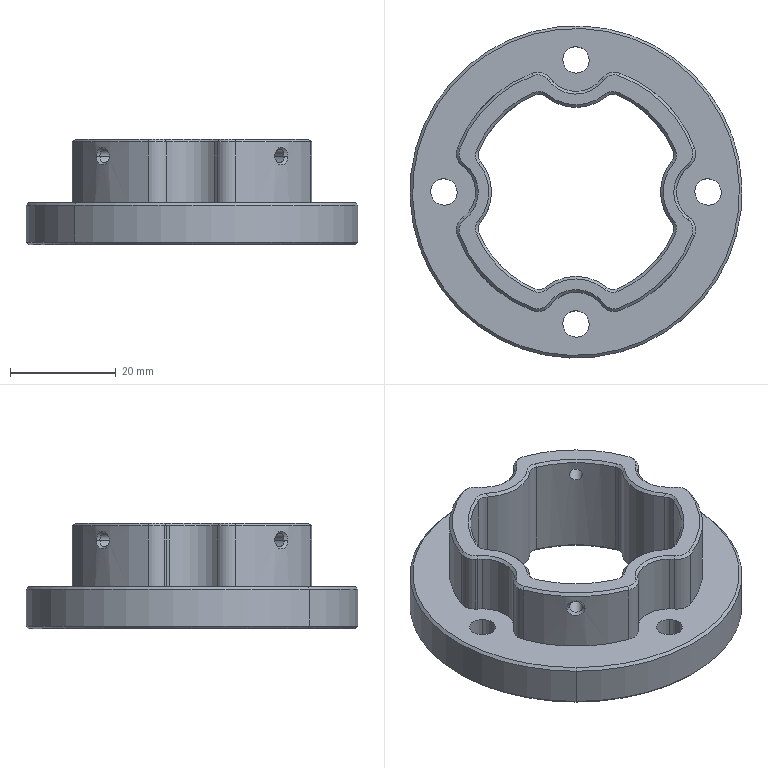NC program | NX | posted with a generic post | part box 62.9 x 62.9 x 20 mm
Whole program:
N10 G17 G21 G94 G90
(FLOOR_WALL_COPY , TOOL : D80)
N12 T19 M6
N14 G54
N16 G17 G0 G90 X-77.45 Y0. S6500 M3
N18 G43 Z30. H19
N20 Z7.
N22 G94 G1 Z4. F1500.
N24 X-71.45
N26 X71.45
N28 X77.45
N30 Z7.
N32 G0 Z30.
N34 X-77.45
N36 Z6.
N38 G1 Z3.
N40 X-71.45
N42 X71.45
N44 X77.45
N46 Z6.
N48 G0 Z30.
N50 X-77.45
N52 Z5.
N54 G1 Z2.
N56 X-71.45
N58 X71.45
N60 X77.45
N62 Z5.
N64 G0 Z30.
N66 X-77.45
N68 Z4.
N70 G1 Z1.
N72 X-71.45
N74 X71.45
N76 X77.45
N78 Z4.
N80 G0 Z30.
N82 X-77.45
N84 Z3.
N86 G1 Z0.
N88 X-71.45
N90 X71.45
N92 X77.45
N94 Z3.
N96 G0 Z30.
N98 M5
(DRILLING_COPY , TOOL : D6A45)
N100 T01 M6
N102 G54
N104 G17 G0 G90 X0. Y-25. S5000 M3
N106 G43 Z30. H1
N108 G94 G81 G98 Z-2.6 F350. R3.
N110 X25. Y0.
N112 X0. Y25.
N114 X-25. Y0.
N116 G80
N118 G0 X-25. Y0. Z30.
(PLANAR_MILL_COPY_COPY_COPY_COPY_COPY_COPY_1_COPY_1 , TOOL : D6A45)
N120 X-32.95 Y-0.866 S9500
N122 Z0.
N124 G1 Z-1.5 F1250.
N126 G3 X-32.45 Y0. R1.
N128 G2 X0. Y32.45 R32.45
N130 X-32.45 Y0. R-32.45
N132 G3 X-32.95 Y0.866 R1.
N134 G1 Z0.
N136 G0 Z30.
N138 X-14.5
N140 Z0.
N142 G1 Z-1.5
N144 G3 X-15. Y0. R1.
N146 G2 X-17.295 Y-6.374 R10.
N148 G3 X-17.445 Y-7.402 R1.
N150 X-7.402 Y-17.445 R18.95
N152 X-6.374 Y-17.295 R1.
N154 G2 X6.374 Y-17.295 R10.
N156 G3 X7.402 Y-17.445 R1.
N158 X17.445 Y-7.402 R18.95
N160 X17.295 Y-6.374 R1.
N162 G2 X17.295 Y6.374 R10.
N164 G3 X17.445 Y7.402 R1.
N166 X7.402 Y17.445 R18.95
N168 X6.374 Y17.295 R1.
N170 G2 X-6.374 Y17.295 R10.
N172 G3 X-7.402 Y17.445 R1.
N174 X-17.445 Y7.402 R18.95
N176 X-17.295 Y6.374 R1.
N178 G2 X-15. Y0. R10.
N180 G3 X-14.5 Y-0.866 R1.
N182 G1 Z0.
N184 G0 Z30.
N186 M5
N188 M2